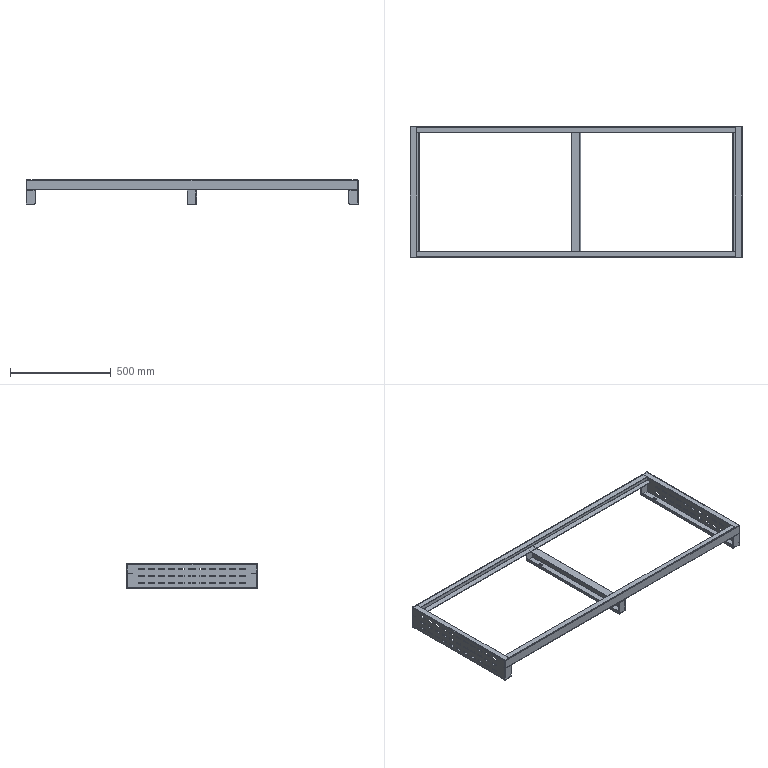Part | SolidWorks | 5 solids | 504 faces | box 1650 x 650 x 120 mm | volume 2092704 mm3 | plane 312 | cylinder 188 | spline 4 | commonest cylinder face diameters 9 x132 0.2 x19 6.2 x19 13 x12 6 x6